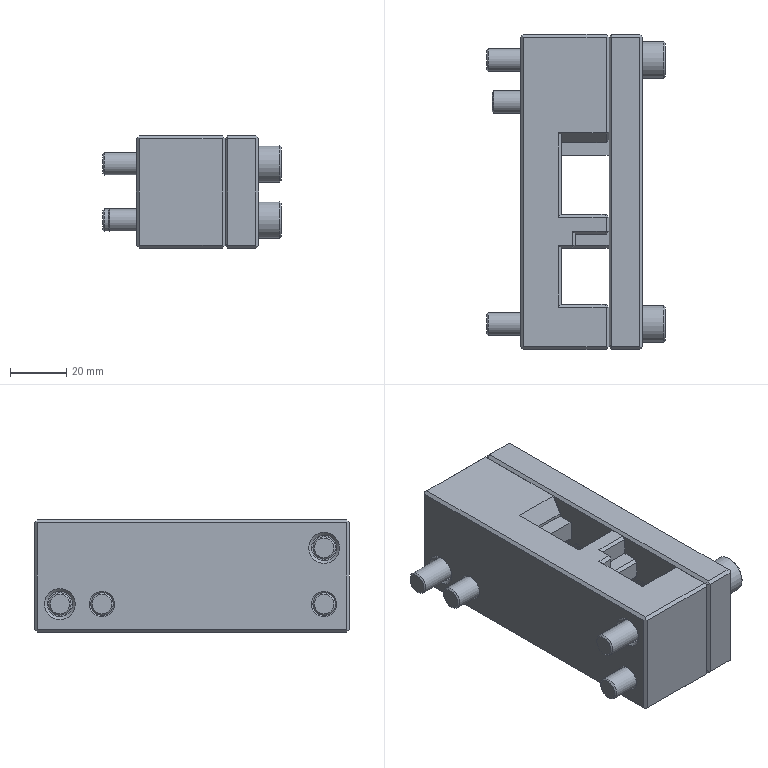Part | NX | features BREP 20, solid 18, CHAMFER 16, SUBTRACT 4 | 9 solids | 407 faces | box 63.5 x 112 x 40 mm | volume 159871 mm3 | plane 241 | spline 112 | cone 34 | cylinder 20 | commonest cylinder face diameters 8 x6 6 x4 9 x4 10.5 x2 12 x2 13 x2